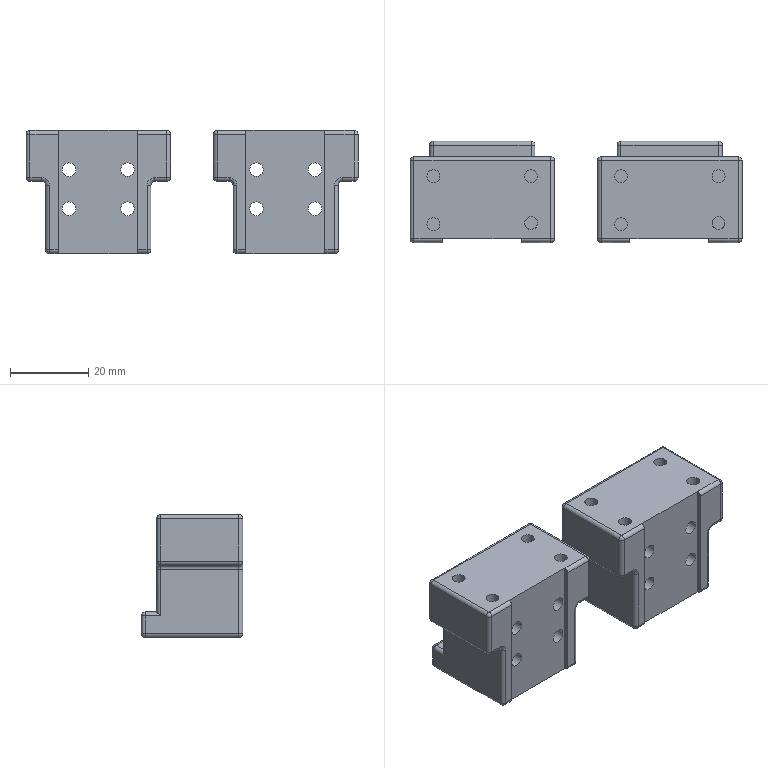CAM job | NX | 3+2 milling, drilling | part box 85 x 26 x 31.5 mm | stock box 90 x 30 x 36.5 mm
Tools:
number,name,description,diameter,corner_radius,flute_length,length,flutes
4,D4,平底铣刀-粗,4.0,0.0,25.0,75.0,2
8,D8,平底铣刀-粗,8.0,0.0,30.0,75.0,2
9,D10,平底铣刀-粗,10.0,0.0,35.0,75.0,2
18,D3-J,平底铣刀-精,3.0,0.0,50.0,75.0,2
11,D4-J,平底铣刀-精,4.0,0.0,50.0,75.0,2
7,D6-J,平底铣刀-精,6.0,0.0,25.0,75.0,2
10,D10-J,平底铣刀-精,10.0,0.0,35.0,75.0,2
1,D80R0.8飞刀,圆鼻刀-粗,80.0,0.8,50.0,75.0,2
1,D80R0.8飞刀-J,圆鼻刀-精,80.0,0.8,50.0,75.0,2
2,D6倒角刀,倒角刀,6.0,0.0,3.0,25.0,2
19,R1,圆球刀,2.0,1.0,6.0,50.0,2
18,M2X0.4,丝锥,1.6,0.0,35.0,50.0,2
17,ZT1.6,钻头,1.6,0.0,35.0,50.0,2
17,ZT3.5,钻头,3.5,0.0,35.0,50.0,2
15,ZT5,钻头,5.0,0.0,35.0,50.0,2
Operations:
program,operation,operation_type,tool,method,geometry_group,spindle_rpm,surface_speed,feed_per_tooth,feed_cut,feed_plunge,cut_length_mm,path_length_mm,cut_time_min,machine_time_min
B,底壁铣飞面一刀开粗_COPY,VolumeBased25DMillingOperation,D80R0.8飞刀,分层开粗-切深K-步距G,W-B,2800.0,703.696,0.5357,3000.0,100.0,1543.224,3033.91,0.5144,0.6635
B,底壁铣飞面一刀精光_COPY,VolumeBased25DMillingOperation,D80R0.8飞刀-J,侧刃精光-切深K-步距G,W-B,4000.0,1005.28,0.125,1000.0,100.0,192.707,228.707,0.1927,0.1963
B,底壁铣分层开粗-中_COPY,VolumeBased25DMillingOperation,D10,分层开粗-切深K-步距G,W-B,8000.0,251.32,0.25,4000.0,100.0,3103.373,3136.921,0.7758,0.7792
B,打点-深0.8_2,Operation,D6倒角刀,NONE,W-B,8000.0,150.796,0.0312,500.0,90.0,21.6,234.239,0.0432,0.0645
B,沉头孔-钻孔0段,Operation,ZT5,NONE,W-B,2800.0,30.788,0.0179,100.0,90.0,124.08,406.441,1.241,1.269
B,盲平孔-M2螺纹底孔,Operation,ZT1.6,NONE,W-B,3000.0,15.08,0.005,30.0,90.0,44.0,189.113,1.467,1.481
B,铣孔开粗D4_1,CylinderMilling,D4,NONE,W-B,8000.0,100.531,0.075,1200.0,100.0,2485.497,3081.578,2.071,2.131
B,铣孔精光D4_1,CylinderMilling,D4-J,精光步距切深关,W-B,8000.0,100.531,0.0312,500.0,100.0,280.253,876.333,0.5605,0.6201
B,等高螺旋爬面_COPY,ZLevelMilling,R1,等高爬面-切深K-步距G,W-B,8000.0,50.266,0.2812,4500.0,100.0,4390.23,4540.266,0.9756,0.9906
B,钻倒角_1,Operation,D6倒角刀,METHOD,W-B,8000.0,150.796,0.0312,500.0,0.0,16.8,141.599,0.0336,0.0461
B,铣倒角_1,PlanarMilling,D6倒角刀,NONE,W-B,8000.0,150.796,0.0312,500.0,100.0,221.725,681.741,0.4435,0.4895
B,盲平孔-攻牙M2.0,Operation,M2X0.4,METHOD,W-B,1000.0,5.027,0.0002,0.4,90.0,34.0,169.113,85.0,85.013
B,底壁铣精光底面-中_COPY,VolumeBased25DMillingOperation,D10-J,精光步距切深关,W-B,7000.0,175.0,0.0536,1500.0,100.0,483.411,516.011,0.3223,0.3255
B,等高精光-中_COPY,ZLevelMilling,D10-J,侧刃精光-切深K-步距G,W-B,8000.0,251.32,0.0625,1000.0,100.0,101.924,237.524,0.1019,0.1155
B,等高精光往复爬面_COPY_COPY,ZLevelMilling,R1,等高爬面-切深K-步距G,W-B,9000.0,56.549,0.2222,4000.0,100.0,5926.36,6376.989,1.482,1.527
A,顶面,FaceMilling,D80R0.8飞刀,侧刃精光-切深K-步距G,W-A,4000.0,1005.31,0.125,1000.0,100.0,179.0,215.0,0.179,0.1826
A,动态开粗D8_COPY,CavityMilling,D8,动态开粗-切深K-步距K,W-A,8000.0,201.062,0.2188,3500.0,100.0,7310.302,7688.371,2.089,2.127
A,底壁粗_1,VolumeBased25DMillingOperation,D8,METHOD,W-A,8000.0,201.062,0.2188,3500.0,100.0,595.599,752.655,0.1702,0.1859
A,打点-深0.8,Operation,D6倒角刀,NONE,W-A,8000.0,150.796,0.0312,500.0,90.0,14.4,181.081,0.0288,0.0455
A,通孔-3-4,Operation,ZT3.5,NONE,W-A,3000.0,32.987,0.02,120.0,90.0,84.332,320.945,0.7028,0.7264
A,外形侧面,ZLevelMilling,D3-J,METHOD,W-A,9000.0,84.823,0.1111,2000.0,80.0,5885.531,6298.021,2.943,2.985
A,等高精光往复爬面_COPY,ZLevelMilling,R1,等高爬面-切深K-步距G,W-A,9000.0,56.549,0.2222,4000.0,100.0,6202.401,6356.45,1.551,1.566
A,仅选体,SurfaceContour,D6倒角刀,METHOD,W-A,8000.0,150.796,0.1875,3000.0,100.0,259.77,743.453,0.0866,0.135
A,底精_1,VolumeBased25DMillingOperation,D6-J,METHOD,W-A,6000.0,113.0,0.2083,1200.0,100.0,326.8,638.778,0.2723,0.3035
A,底侧精_3,VolumeBased25DMillingOperation,D6-J,METHOD,W-A,6000.0,113.0,0.2083,1200.0,100.0,164.977,388.94,0.1375,0.1599
A,外形半精_2,VolumeBased25DMillingOperation,D6-J,METHOD,W-A,8000.0,251.327,0.0625,1000.0,100.0,622.562,986.882,0.6226,0.659